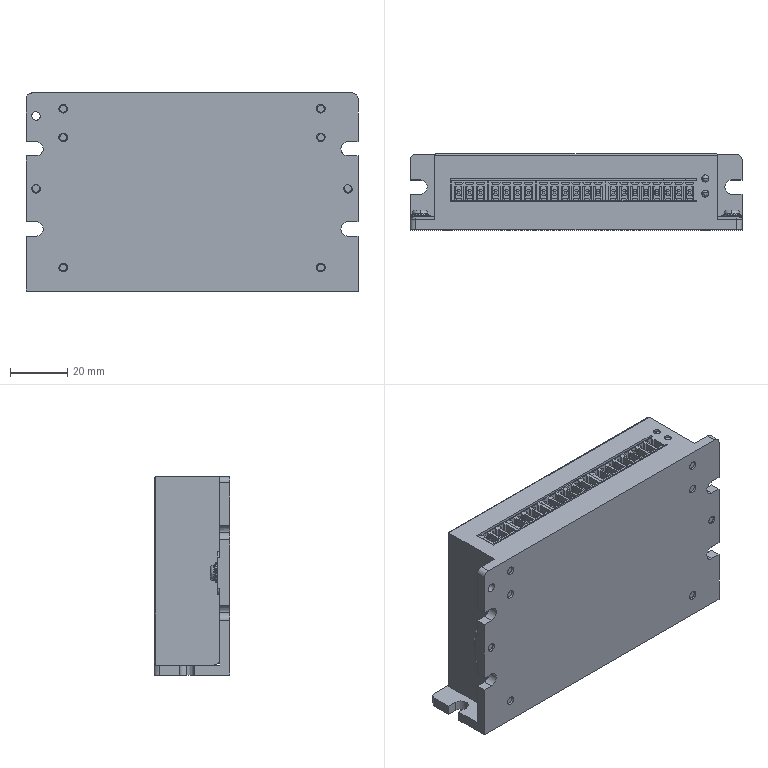Part | STEP file | cl57 | 7 solids | 1501 faces | box 116 x 26.5 x 69.2 mm | volume 66136 mm3 | spline 1501